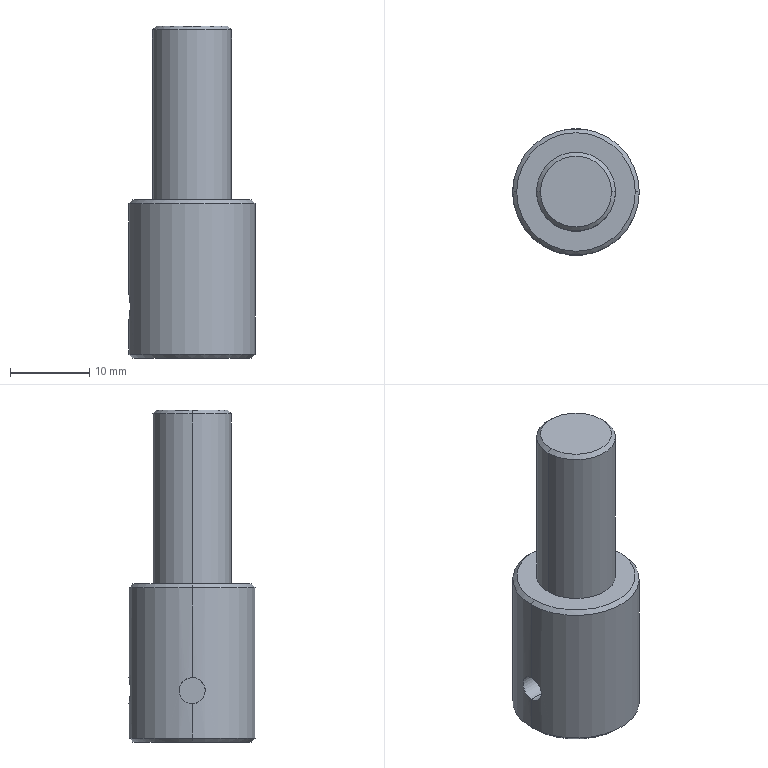Part | STEP file | (PA01.001.LX009) Connecting Shaft | 1 solid | 26 faces | box 16 x 16 x 42 mm | volume 4893 mm3 | plane 12 | cylinder 8 | cone 6 | commonest cylinder face diameters 3.3 x4 10 x2 16 x2